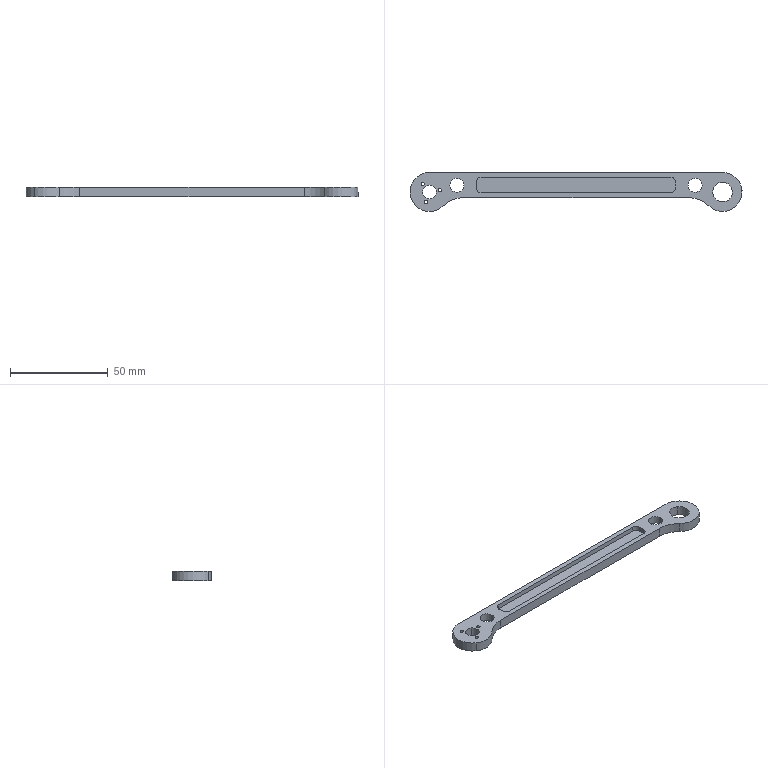Part | NX | features BREP 1 | 1 solid | 43 faces | box 169.999 x 20 x 5 mm | volume 8700 mm3 | cylinder 33 | plane 10 | commonest cylinder face diameters 1.7 x6 5 x6 10 x6 20 x6 7.2 x4 7 x2
STEP:
#1=CARTESIAN_POINT('',(-8.148,-15.081,-8.));
#2=VERTEX_POINT('',#1);
#3=CARTESIAN_POINT('',(-9.848,-15.081,-8.));
#4=VERTEX_POINT('',#3);
#5=CARTESIAN_POINT('',(-8.998,-15.081,-8.));
#6=DIRECTION('',(0.,0.,-1.));
#7=DIRECTION('',(-1.,0.,0.));
#8=AXIS2_PLACEMENT_3D('',#5,#6,#7);
#9=CIRCLE('',#8,0.85);
#10=EDGE_CURVE('',#2,#4,#9,.T.);
#11=ORIENTED_EDGE('',*,*,#10,.T.);
#12=CARTESIAN_POINT('',(-9.848,-15.081,-3.));
#13=VERTEX_POINT('',#12);
#14=CARTESIAN_POINT('',(-9.848,-15.081,-13.));
#15=DIRECTION('',(0.,0.,1.));
#16=VECTOR('',#15,1000.);
#17=LINE('',#14,#16);
#18=EDGE_CURVE('',#4,#13,#17,.T.);
#19=ORIENTED_EDGE('',*,*,#18,.T.);
#20=CARTESIAN_POINT('',(-8.148,-15.081,-3.));
#21=VERTEX_POINT('',#20);
#22=CARTESIAN_POINT('',(-8.998,-15.081,-3.));
#23=DIRECTION('',(0.,0.,1.));
#24=DIRECTION('',(1.,0.,0.));
#25=AXIS2_PLACEMENT_3D('',#22,#23,#24);
#26=CIRCLE('',#25,0.85);
#27=EDGE_CURVE('',#13,#21,#26,.T.);
#28=ORIENTED_EDGE('',*,*,#27,.T.);
#29=CARTESIAN_POINT('',(-8.148,-15.081,-13.));
#30=DIRECTION('',(0.,0.,1.));
#31=VECTOR('',#30,1000.);
#32=LINE('',#29,#31);
#33=EDGE_CURVE('',#2,#21,#32,.T.);
#34=ORIENTED_EDGE('',*,*,#33,.F.);
#35=EDGE_LOOP('',(#11,#19,#28,#34));
#36=FACE_BOUND('',#35,.T.);
#37=CARTESIAN_POINT('',(-8.998,-15.081,-13.));
#38=DIRECTION('',(0.,0.,1.));
#39=DIRECTION('',(-1.,0.,0.));
#40=AXIS2_PLACEMENT_3D('',#37,#38,#39);
#41=CYLINDRICAL_SURFACE('',#40,0.85);
#42=ADVANCED_FACE('',(#36),#41,.F.);
#43=CARTESIAN_POINT('',(-9.816,-5.882,-8.));
#44=VERTEX_POINT('',#43);
#45=CARTESIAN_POINT('',(-11.516,-5.882,-8.));
#46=VERTEX_POINT('',#45);
#47=CARTESIAN_POINT('',(-10.666,-5.882,-8.));
#48=DIRECTION('',(0.,0.,-1.));
#49=DIRECTION('',(-1.,0.,0.));
#50=AXIS2_PLACEMENT_3D('',#47,#48,#49);
#51=CIRCLE('',#50,0.85);
#52=EDGE_CURVE('',#44,#46,#51,.T.);
#53=ORIENTED_EDGE('',*,*,#52,.T.);
#54=CARTESIAN_POINT('',(-11.516,-5.882,-3.));
#55=VERTEX_POINT('',#54);
#56=CARTESIAN_POINT('',(-11.516,-5.882,-13.));
#57=DIRECTION('',(0.,0.,1.));
#58=VECTOR('',#57,1000.);
#59=LINE('',#56,#58);
#60=EDGE_CURVE('',#46,#55,#59,.T.);
#61=ORIENTED_EDGE('',*,*,#60,.T.);
#62=CARTESIAN_POINT('',(-9.816,-5.882,-3.));
#63=VERTEX_POINT('',#62);
#64=CARTESIAN_POINT('',(-10.666,-5.882,-3.));
#65=DIRECTION('',(0.,0.,1.));
#66=DIRECTION('',(1.,0.,0.));
#67=AXIS2_PLACEMENT_3D('',#64,#65,#66);
#68=CIRCLE('',#67,0.85);
#69=EDGE_CURVE('',#55,#63,#68,.T.);
#70=ORIENTED_EDGE('',*,*,#69,.T.);
#71=CARTESIAN_POINT('',(-9.816,-5.882,-13.));
#72=DIRECTION('',(0.,0.,1.));
#73=VECTOR('',#72,1000.);
#74=LINE('',#71,#73);
#75=EDGE_CURVE('',#44,#63,#74,.T.);
#76=ORIENTED_EDGE('',*,*,#75,.F.);
#77=EDGE_LOOP('',(#53,#61,#70,#76));
#78=FACE_BOUND('',#77,.T.);
#79=CARTESIAN_POINT('',(-10.666,-5.882,-13.));
#80=DIRECTION('',(0.,0.,1.));
#81=DIRECTION('',(-1.,0.,0.));
#82=AXIS2_PLACEMENT_3D('',#79,#80,#81);
#83=CYLINDRICAL_SURFACE('',#82,0.85);
#84=ADVANCED_FACE('',(#78),#83,.F.);
#85=CARTESIAN_POINT('',(-1.015,-9.037,-8.));
#86=VERTEX_POINT('',#85);
#87=CARTESIAN_POINT('',(-2.715,-9.037,-8.));
#88=VERTEX_POINT('',#87);
#89=CARTESIAN_POINT('',(-1.865,-9.037,-8.));
#90=DIRECTION('',(0.,0.,-1.));
#91=DIRECTION('',(-1.,0.,0.));
#92=AXIS2_PLACEMENT_3D('',#89,#90,#91);
#93=CIRCLE('',#92,0.85);
#94=EDGE_CURVE('',#86,#88,#93,.T.);
#95=ORIENTED_EDGE('',*,*,#94,.T.);
#96=CARTESIAN_POINT('',(-2.715,-9.037,-3.));
#97=VERTEX_POINT('',#96);
#98=CARTESIAN_POINT('',(-2.715,-9.037,-13.));
#99=DIRECTION('',(0.,0.,1.));
#100=VECTOR('',#99,1000.);
#101=LINE('',#98,#100);
#102=EDGE_CURVE('',#88,#97,#101,.T.);
#103=ORIENTED_EDGE('',*,*,#102,.T.);
#104=CARTESIAN_POINT('',(-1.015,-9.037,-3.));
#105=VERTEX_POINT('',#104);
#106=CARTESIAN_POINT('',(-1.865,-9.037,-3.));
#107=DIRECTION('',(0.,0.,1.));
#108=DIRECTION('',(1.,0.,0.));
#109=AXIS2_PLACEMENT_3D('',#106,#107,#108);
#110=CIRCLE('',#109,0.85);
#111=EDGE_CURVE('',#97,#105,#110,.T.);
#112=ORIENTED_EDGE('',*,*,#111,.T.);
#113=CARTESIAN_POINT('',(-1.015,-9.037,-13.));
#114=DIRECTION('',(0.,0.,1.));
#115=VECTOR('',#114,1000.);
#116=LINE('',#113,#115);
#117=EDGE_CURVE('',#86,#105,#116,.T.);
#118=ORIENTED_EDGE('',*,*,#117,.F.);
#119=EDGE_LOOP('',(#95,#103,#112,#118));
#120=FACE_BOUND('',#119,.T.);
#121=CARTESIAN_POINT('',(-1.865,-9.037,-13.));
#122=DIRECTION('',(0.,0.,1.));
#123=DIRECTION('',(-1.,0.,0.));
#124=AXIS2_PLACEMENT_3D('',#121,#122,#123);
#125=CYLINDRICAL_SURFACE('',#124,0.85);
#126=ADVANCED_FACE('',(#120),#125,.F.);
#127=CARTESIAN_POINT('',(16.824,-6.577,-5.5));
#128=VERTEX_POINT('',#127);
#129=CARTESIAN_POINT('',(16.771,-7.608,-5.5));
#130=VERTEX_POINT('',#129);
#131=CARTESIAN_POINT('',(6.824,-6.577,-5.5));
#132=DIRECTION('',(0.,0.,-1.));
#133=DIRECTION('',(1.,0.,0.));
#134=AXIS2_PLACEMENT_3D('',#131,#132,#133);
#135=CIRCLE('',#134,10.);
#136=EDGE_CURVE('',#128,#130,#135,.T.);
#137=ORIENTED_EDGE('',*,*,#136,.F.);
#138=CARTESIAN_POINT('',(16.824,-6.577,-3.));
#139=VERTEX_POINT('',#138);
#140=CARTESIAN_POINT('',(16.824,-6.577,-5.5));
#141=DIRECTION('',(0.,0.,1.));
#142=VECTOR('',#141,1000.);
#143=LINE('',#140,#142);
#144=EDGE_CURVE('',#128,#139,#143,.T.);
#145=ORIENTED_EDGE('',*,*,#144,.T.);
#146=CARTESIAN_POINT('',(16.771,-7.608,-3.));
#147=VERTEX_POINT('',#146);
#148=CARTESIAN_POINT('',(6.824,-6.577,-3.));
#149=DIRECTION('',(0.,0.,-1.));
#150=DIRECTION('',(1.,0.,0.));
#151=AXIS2_PLACEMENT_3D('',#148,#149,#150);
#152=CIRCLE('',#151,10.);
#153=EDGE_CURVE('',#139,#147,#152,.T.);
#154=ORIENTED_EDGE('',*,*,#153,.T.);
#155=CARTESIAN_POINT('',(16.771,-7.608,-5.5));
#156=DIRECTION('',(0.,0.,1.));
#157=VECTOR('',#156,1000.);
#158=LINE('',#155,#157);
#159=EDGE_CURVE('',#130,#147,#158,.T.);
#160=ORIENTED_EDGE('',*,*,#159,.F.);
#161=EDGE_LOOP('',(#137,#145,#154,#160));
#162=FACE_BOUND('',#161,.T.);
#163=CARTESIAN_POINT('',(6.824,-6.577,-5.5));
#164=DIRECTION('',(0.,0.,1.));
#165=DIRECTION('',(-1.,0.,0.));
#166=AXIS2_PLACEMENT_3D('',#163,#164,#165);
#167=CYLINDRICAL_SURFACE('',#166,10.);
#168=ADVANCED_FACE('',(#162),#167,.T.);
#169=CARTESIAN_POINT('',(118.89,-7.866,-5.5));
#170=VERTEX_POINT('',#169);
#171=CARTESIAN_POINT('',(118.877,-7.608,-5.5));
#172=VERTEX_POINT('',#171);
#173=CARTESIAN_POINT('',(116.39,-7.866,-5.5));
#174=DIRECTION('',(0.,0.,1.));
#175=DIRECTION('',(1.,0.,0.));
#176=AXIS2_PLACEMENT_3D('',#173,#174,#175);
#177=CIRCLE('',#176,2.5);
#178=EDGE_CURVE('',#170,#172,#177,.T.);
#179=ORIENTED_EDGE('',*,*,#178,.F.);
#180=CARTESIAN_POINT('',(118.89,-7.866,-3.));
#181=VERTEX_POINT('',#180);
#182=CARTESIAN_POINT('',(118.89,-7.866,-5.5));
#183=DIRECTION('',(0.,0.,1.));
#184=VECTOR('',#183,1000.);
#185=LINE('',#182,#184);
#186=EDGE_CURVE('',#170,#181,#185,.T.);
#187=ORIENTED_EDGE('',*,*,#186,.T.);
#188=CARTESIAN_POINT('',(118.877,-7.608,-3.));
#189=VERTEX_POINT('',#188);
#190=CARTESIAN_POINT('',(116.39,-7.866,-3.));
#191=DIRECTION('',(0.,0.,1.));
#192=DIRECTION('',(1.,0.,0.));
#193=AXIS2_PLACEMENT_3D('',#190,#191,#192);
#194=CIRCLE('',#193,2.5);
#195=EDGE_CURVE('',#181,#189,#194,.T.);
#196=ORIENTED_EDGE('',*,*,#195,.T.);
#197=CARTESIAN_POINT('',(118.877,-7.608,-5.5));
#198=DIRECTION('',(0.,0.,1.));
#199=VECTOR('',#198,1000.);
#200=LINE('',#197,#199);
#201=EDGE_CURVE('',#172,#189,#200,.T.);
#202=ORIENTED_EDGE('',*,*,#201,.F.);
#203=EDGE_LOOP('',(#179,#187,#196,#202));
#204=FACE_BOUND('',#203,.T.);
#205=CARTESIAN_POINT('',(116.39,-7.866,-5.5));
#206=DIRECTION('',(0.,0.,1.));
#207=DIRECTION('',(-1.,0.,0.));
#208=AXIS2_PLACEMENT_3D('',#205,#206,#207);
#209=CYLINDRICAL_SURFACE('',#208,2.5);
#210=ADVANCED_FACE('',(#204),#209,.F.);
#211=CARTESIAN_POINT('',(118.924,-5.,-5.5));
#212=VERTEX_POINT('',#211);
#213=CARTESIAN_POINT('',(116.424,-2.5,-5.5));
#214=VERTEX_POINT('',#213);
#215=CARTESIAN_POINT('',(116.424,-5.,-5.5));
#216=DIRECTION('',(0.,0.,1.));
#217=DIRECTION('',(1.,0.,0.));
#218=AXIS2_PLACEMENT_3D('',#215,#216,#217);
#219=CIRCLE('',#218,2.5);
#220=EDGE_CURVE('',#212,#214,#219,.T.);
#221=ORIENTED_EDGE('',*,*,#220,.F.);
#222=CARTESIAN_POINT('',(118.924,-5.,-3.));
#223=VERTEX_POINT('',#222);
#224=CARTESIAN_POINT('',(118.924,-5.,-5.5));
#225=DIRECTION('',(0.,0.,1.));
#226=VECTOR('',#225,1000.);
#227=LINE('',#224,#226);
#228=EDGE_CURVE('',#212,#223,#227,.T.);
#229=ORIENTED_EDGE('',*,*,#228,.T.);
#230=CARTESIAN_POINT('',(116.424,-2.5,-3.));
#231=VERTEX_POINT('',#230);
#232=CARTESIAN_POINT('',(116.424,-5.,-3.));
#233=DIRECTION('',(0.,0.,1.));
#234=DIRECTION('',(1.,0.,0.));
#235=AXIS2_PLACEMENT_3D('',#232,#233,#234);
#236=CIRCLE('',#235,2.5);
#237=EDGE_CURVE('',#223,#231,#236,.T.);
#238=ORIENTED_EDGE('',*,*,#237,.T.);
#239=CARTESIAN_POINT('',(116.424,-2.5,-5.5));
#240=DIRECTION('',(0.,0.,1.));
#241=VECTOR('',#240,1000.);
#242=LINE('',#239,#241);
#243=EDGE_CURVE('',#214,#231,#242,.T.);
#244=ORIENTED_EDGE('',*,*,#243,.F.);
#245=EDGE_LOOP('',(#221,#229,#238,#244));
#246=FACE_BOUND('',#245,.T.);
#247=CARTESIAN_POINT('',(116.424,-5.,-5.5));
#248=DIRECTION('',(0.,0.,1.));
#249=DIRECTION('',(-1.,0.,0.));
#250=AXIS2_PLACEMENT_3D('',#247,#248,#249);
#251=CYLINDRICAL_SURFACE('',#250,2.5);
#252=ADVANCED_FACE('',(#246),#251,.F.);
#253=CARTESIAN_POINT('',(11.824,-6.577,-7.));
#254=VERTEX_POINT('',#253);
#255=CARTESIAN_POINT('',(1.824,-6.577,-7.));
#256=VERTEX_POINT('',#255);
#257=CARTESIAN_POINT('',(6.824,-6.577,-7.));
#258=DIRECTION('',(0.,0.,-1.));
#259=DIRECTION('',(-1.,0.,0.));
#260=AXIS2_PLACEMENT_3D('',#257,#258,#259);
#261=CIRCLE('',#260,5.);
#262=EDGE_CURVE('',#254,#256,#261,.T.);
#263=ORIENTED_EDGE('',*,*,#262,.F.);
#264=CARTESIAN_POINT('',(11.824,-6.577,-8.));
#265=VERTEX_POINT('',#264);
#266=CARTESIAN_POINT('',(11.824,-6.577,-7.));
#267=DIRECTION('',(0.,0.,-1.));
#268=VECTOR('',#267,1000.);
#269=LINE('',#266,#268);
#270=EDGE_CURVE('',#265,#254,#269,.F.);
#271=ORIENTED_EDGE('',*,*,#270,.F.);
#272=CARTESIAN_POINT('',(1.824,-6.577,-8.));
#273=VERTEX_POINT('',#272);
#274=CARTESIAN_POINT('',(6.824,-6.577,-8.));
#275=DIRECTION('',(0.,0.,-1.));
#276=DIRECTION('',(-1.,0.,0.));
#277=AXIS2_PLACEMENT_3D('',#274,#275,#276);
#278=CIRCLE('',#277,5.);
#279=EDGE_CURVE('',#265,#273,#278,.T.);
#280=ORIENTED_EDGE('',*,*,#279,.T.);
#281=CARTESIAN_POINT('',(1.824,-6.577,-7.));
#282=DIRECTION('',(0.,0.,-1.));
#283=VECTOR('',#282,1000.);
#284=LINE('',#281,#283);
#285=EDGE_CURVE('',#273,#256,#284,.F.);
#286=ORIENTED_EDGE('',*,*,#285,.T.);
#287=EDGE_LOOP('',(#263,#271,#280,#286));
#288=FACE_BOUND('',#287,.T.);
#289=CARTESIAN_POINT('',(6.824,-6.577,-7.));
#290=DIRECTION('',(0.,0.,-1.));
#291=DIRECTION('',(1.,0.,0.));
#292=AXIS2_PLACEMENT_3D('',#289,#290,#291);
#293=CYLINDRICAL_SURFACE('',#292,5.);
#294=ADVANCED_FACE('',(#288),#293,.F.);
#295=CARTESIAN_POINT('',(133.824,-6.577,-7.));
#296=VERTEX_POINT('',#295);
#297=CARTESIAN_POINT('',(123.824,-6.577,-7.));
#298=VERTEX_POINT('',#297);
#299=CARTESIAN_POINT('',(128.824,-6.577,-7.));
#300=DIRECTION('',(0.,0.,-1.));
#301=DIRECTION('',(-1.,0.,0.));
#302=AXIS2_PLACEMENT_3D('',#299,#300,#301);
#303=CIRCLE('',#302,5.);
#304=EDGE_CURVE('',#296,#298,#303,.T.);
#305=ORIENTED_EDGE('',*,*,#304,.F.);
#306=CARTESIAN_POINT('',(133.824,-6.577,-8.));
#307=VERTEX_POINT('',#306);
#308=CARTESIAN_POINT('',(133.824,-6.577,-7.));
#309=DIRECTION('',(0.,0.,-1.));
#310=VECTOR('',#309,1000.);
#311=LINE('',#308,#310);
#312=EDGE_CURVE('',#307,#296,#311,.F.);
#313=ORIENTED_EDGE('',*,*,#312,.F.);
#314=CARTESIAN_POINT('',(123.824,-6.577,-8.));
#315=VERTEX_POINT('',#314);
#316=CARTESIAN_POINT('',(128.824,-6.577,-8.));
#317=DIRECTION('',(0.,0.,-1.));
#318=DIRECTION('',(-1.,0.,0.));
#319=AXIS2_PLACEMENT_3D('',#316,#317,#318);
#320=CIRCLE('',#319,5.);
#321=EDGE_CURVE('',#307,#315,#320,.T.);
#322=ORIENTED_EDGE('',*,*,#321,.T.);
#323=CARTESIAN_POINT('',(123.824,-6.577,-7.));
#324=DIRECTION('',(0.,0.,-1.));
#325=VECTOR('',#324,1000.);
#326=LINE('',#323,#325);
#327=EDGE_CURVE('',#315,#298,#326,.F.);
#328=ORIENTED_EDGE('',*,*,#327,.T.);
#329=EDGE_LOOP('',(#305,#313,#322,#328));
#330=FACE_BOUND('',#329,.T.);
#331=CARTESIAN_POINT('',(128.824,-6.577,-7.));
#332=DIRECTION('',(0.,0.,-1.));
#333=DIRECTION('',(1.,0.,0.));
#334=AXIS2_PLACEMENT_3D('',#331,#332,#333);
#335=CYLINDRICAL_SURFACE('',#334,5.);
#336=ADVANCED_FACE('',(#330),#335,.F.);
#337=CARTESIAN_POINT('',(145.634,-5.864,-8.));
#338=VERTEX_POINT('',#337);
#339=CARTESIAN_POINT('',(140.014,-14.136,-8.));
#340=VERTEX_POINT('',#339);
#341=CARTESIAN_POINT('',(142.824,-10.,-8.));
#342=DIRECTION('',(0.,0.,1.));
#343=DIRECTION('',(-1.,0.,0.));
#344=AXIS2_PLACEMENT_3D('',#341,#342,#343);
#345=CIRCLE('',#344,5.);
#346=EDGE_CURVE('',#338,#340,#345,.T.);
#347=ORIENTED_EDGE('',*,*,#346,.F.);
#348=CARTESIAN_POINT('',(145.634,-5.864,-3.));
#349=VERTEX_POINT('',#348);
#350=CARTESIAN_POINT('',(145.634,-5.864,-6.));
#351=DIRECTION('',(0.,0.,1.));
#352=VECTOR('',#351,1000.);
#353=LINE('',#350,#352);
#354=EDGE_CURVE('',#349,#338,#353,.F.);
#355=ORIENTED_EDGE('',*,*,#354,.F.);
#356=CARTESIAN_POINT('',(140.014,-14.136,-3.));
#357=VERTEX_POINT('',#356);
#358=CARTESIAN_POINT('',(142.824,-10.,-3.));
#359=DIRECTION('',(0.,0.,1.));
#360=DIRECTION('',(-1.,0.,0.));
#361=AXIS2_PLACEMENT_3D('',#358,#359,#360);
#362=CIRCLE('',#361,5.);
#363=EDGE_CURVE('',#349,#357,#362,.T.);
#364=ORIENTED_EDGE('',*,*,#363,.T.);
#365=CARTESIAN_POINT('',(140.014,-14.136,-6.));
#366=DIRECTION('',(0.,0.,1.));
#367=VECTOR('',#366,1000.);
#368=LINE('',#365,#367);
#369=EDGE_CURVE('',#357,#340,#368,.F.);
#370=ORIENTED_EDGE('',*,*,#369,.T.);
#371=EDGE_LOOP('',(#347,#355,#364,#370));
#372=FACE_BOUND('',#371,.T.);
#373=CARTESIAN_POINT('',(142.824,-10.,-6.));
#374=DIRECTION('',(0.,0.,1.));
#375=DIRECTION('',(0.562,0.8271,0.));
#376=AXIS2_PLACEMENT_3D('',#373,#374,#375);
#377=CYLINDRICAL_SURFACE('',#376,5.);
#378=ADVANCED_FACE('',(#372),#377,.F.);
#379=CARTESIAN_POINT('',(-7.176,0.,-8.));
#380=VERTEX_POINT('',#379);
#381=CARTESIAN_POINT('',(-12.797,-18.271,-8.));
#382=VERTEX_POINT('',#381);
#383=CARTESIAN_POINT('',(-7.176,-10.,-8.));
#384=DIRECTION('',(0.,0.,1.));
#385=DIRECTION('',(-1.,0.,0.));
#386=AXIS2_PLACEMENT_3D('',#383,#384,#385);
#387=CIRCLE('',#386,10.);
#388=EDGE_CURVE('',#380,#382,#387,.T.);
#389=ORIENTED_EDGE('',*,*,#388,.T.);
#390=CARTESIAN_POINT('',(-12.797,-18.271,-3.));
#391=VERTEX_POINT('',#390);
#392=CARTESIAN_POINT('',(-12.797,-18.271,-6.));
#393=DIRECTION('',(0.,0.,1.));
#394=VECTOR('',#393,1000.);
#395=LINE('',#392,#394);
#396=EDGE_CURVE('',#382,#391,#395,.T.);
#397=ORIENTED_EDGE('',*,*,#396,.T.);
#398=CARTESIAN_POINT('',(-7.176,0.,-3.));
#399=VERTEX_POINT('',#398);
#400=CARTESIAN_POINT('',(-7.176,-10.,-3.));
#401=DIRECTION('',(0.,0.,1.));
#402=DIRECTION('',(0.562,0.8271,0.));
#403=AXIS2_PLACEMENT_3D('',#400,#401,#402);
#404=CIRCLE('',#403,10.);
#405=EDGE_CURVE('',#399,#391,#404,.T.);
#406=ORIENTED_EDGE('',*,*,#405,.F.);
#407=CARTESIAN_POINT('',(-7.176,0.,-6.));
#408=DIRECTION('',(0.,0.,1.));
#409=VECTOR('',#408,1000.);
#410=LINE('',#407,#409);
#411=EDGE_CURVE('',#380,#399,#410,.T.);
#412=ORIENTED_EDGE('',*,*,#411,.F.);
#413=EDGE_LOOP('',(#389,#397,#406,#412));
#414=FACE_BOUND('',#413,.T.);
#415=CARTESIAN_POINT('',(-7.176,-10.,-6.));
#416=DIRECTION('',(0.,0.,1.));
#417=DIRECTION('',(0.562,0.8271,0.));
#418=AXIS2_PLACEMENT_3D('',#415,#416,#417);
#419=CYLINDRICAL_SURFACE('',#418,10.);
#420=ADVANCED_FACE('',(#414),#419,.T.);
#421=CARTESIAN_POINT('',(-5.209,-7.105,-8.));
#422=VERTEX_POINT('',#421);
#423=CARTESIAN_POINT('',(-9.143,-12.895,-8.));
#424=VERTEX_POINT('',#423);
#425=CARTESIAN_POINT('',(-7.176,-10.,-8.));
#426=DIRECTION('',(0.,0.,1.));
#427=DIRECTION('',(-1.,0.,0.));
#428=AXIS2_PLACEMENT_3D('',#425,#426,#427);
#429=CIRCLE('',#428,3.5);
#430=EDGE_CURVE('',#422,#424,#429,.T.);
#431=ORIENTED_EDGE('',*,*,#430,.F.);
#432=CARTESIAN_POINT('',(-5.209,-7.105,-3.));
#433=VERTEX_POINT('',#432);
#434=CARTESIAN_POINT('',(-5.209,-7.105,-6.));
#435=DIRECTION('',(0.,0.,1.));
#436=VECTOR('',#435,1000.);
#437=LINE('',#434,#436);
#438=EDGE_CURVE('',#433,#422,#437,.F.);
#439=ORIENTED_EDGE('',*,*,#438,.F.);
#440=CARTESIAN_POINT('',(-9.143,-12.895,-3.));
#441=VERTEX_POINT('',#440);
#442=CARTESIAN_POINT('',(-7.176,-10.,-3.));
#443=DIRECTION('',(0.,0.,1.));
#444=DIRECTION('',(-1.,0.,0.));
#445=AXIS2_PLACEMENT_3D('',#442,#443,#444);
#446=CIRCLE('',#445,3.5);
#447=EDGE_CURVE('',#433,#441,#446,.T.);
#448=ORIENTED_EDGE('',*,*,#447,.T.);
#449=CARTESIAN_POINT('',(-9.143,-12.895,-6.));
#450=DIRECTION('',(0.,0.,1.));
#451=VECTOR('',#450,1000.);
#452=LINE('',#449,#451);
#453=EDGE_CURVE('',#441,#424,#452,.F.);
#454=ORIENTED_EDGE('',*,*,#453,.T.);
#455=EDGE_LOOP('',(#431,#439,#448,#454));
#456=FACE_BOUND('',#455,.T.);
#457=CARTESIAN_POINT('',(-7.176,-10.,-6.));
#458=DIRECTION('',(0.,0.,1.));
#459=DIRECTION('',(0.562,0.8271,0.));
#460=AXIS2_PLACEMENT_3D('',#457,#458,#459);
#461=CYLINDRICAL_SURFACE('',#460,3.5);
#462=ADVANCED_FACE('',(#456),#461,.F.);
#463=CARTESIAN_POINT('',(132.424,-6.577,-3.));
#464=VERTEX_POINT('',#463);
#465=CARTESIAN_POINT('',(125.224,-6.577,-3.));
#466=VERTEX_POINT('',#465);
#467=CARTESIAN_POINT('',(128.824,-6.577,-3.));
#468=DIRECTION('',(0.,0.,-1.));
#469=DIRECTION('',(-1.,0.,0.));
#470=AXIS2_PLACEMENT_3D('',#467,#468,#469);
#471=CIRCLE('',#470,3.6);
#472=EDGE_CURVE('',#464,#466,#471,.T.);
#473=ORIENTED_EDGE('',*,*,#472,.F.);
#474=CARTESIAN_POINT('',(132.424,-6.577,-7.));
#475=VERTEX_POINT('',#474);
#476=CARTESIAN_POINT('',(132.424,-6.577,28.));
#477=DIRECTION('',(0.,0.,-1.));
#478=VECTOR('',#477,1000.);
#479=LINE('',#476,#478);
#480=EDGE_CURVE('',#475,#464,#479,.F.);
#481=ORIENTED_EDGE('',*,*,#480,.F.);
#482=CARTESIAN_POINT('',(125.224,-6.577,-7.));
#483=VERTEX_POINT('',#482);
#484=CARTESIAN_POINT('',(128.824,-6.577,-7.));
#485=DIRECTION('',(0.,0.,1.));
#486=DIRECTION('',(-1.,0.,0.));
#487=AXIS2_PLACEMENT_3D('',#484,#485,#486);
#488=CIRCLE('',#487,3.6);
#489=EDGE_CURVE('',#483,#475,#488,.T.);
#490=ORIENTED_EDGE('',*,*,#489,.F.);
#491=CARTESIAN_POINT('',(125.224,-6.577,28.));
#492=DIRECTION('',(0.,0.,-1.));
#493=VECTOR('',#492,1000.);
#494=LINE('',#491,#493);
#495=EDGE_CURVE('',#483,#466,#494,.F.);
#496=ORIENTED_EDGE('',*,*,#495,.T.);
#497=EDGE_LOOP('',(#473,#481,#490,#496));
#498=FACE_BOUND('',#497,.T.);
#499=CARTESIAN_POINT('',(128.824,-6.577,28.));
#500=DIRECTION('',(0.,0.,-1.));
#501=DIRECTION('',(1.,0.,0.));
#502=AXIS2_PLACEMENT_3D('',#499,#500,#501);
#503=CYLINDRICAL_SURFACE('',#502,3.6);
#504=ADVANCED_FACE('',(#498),#503,.F.);
#505=CARTESIAN_POINT('',(10.424,-6.577,-3.));
#506=VERTEX_POINT('',#505);
#507=CARTESIAN_POINT('',(3.224,-6.577,-3.));
#508=VERTEX_POINT('',#507);
#509=CARTESIAN_POINT('',(6.824,-6.577,-3.));
#510=DIRECTION('',(0.,0.,-1.));
#511=DIRECTION('',(-1.,0.,0.));
#512=AXIS2_PLACEMENT_3D('',#509,#510,#511);
#513=CIRCLE('',#512,3.6);
#514=EDGE_CURVE('',#506,#508,#513,.T.);
#515=ORIENTED_EDGE('',*,*,#514,.F.);
#516=CARTESIAN_POINT('',(10.424,-6.577,-7.));
#517=VERTEX_POINT('',#516);
#518=CARTESIAN_POINT('',(10.424,-6.577,28.));
#519=DIRECTION('',(0.,0.,-1.));
#520=VECTOR('',#519,1000.);
#521=LINE('',#518,#520);
#522=EDGE_CURVE('',#517,#506,#521,.F.);
#523=ORIENTED_EDGE('',*,*,#522,.F.);
#524=CARTESIAN_POINT('',(3.224,-6.577,-7.));
#525=VERTEX_POINT('',#524);
#526=CARTESIAN_POINT('',(6.824,-6.577,-7.));
#527=DIRECTION('',(0.,0.,1.));
#528=DIRECTION('',(-1.,0.,0.));
#529=AXIS2_PLACEMENT_3D('',#526,#527,#528);
#530=CIRCLE('',#529,3.6);
#531=EDGE_CURVE('',#525,#517,#530,.T.);
#532=ORIENTED_EDGE('',*,*,#531,.F.);
#533=CARTESIAN_POINT('',(3.224,-6.577,28.));
#534=DIRECTION('',(0.,0.,-1.));
#535=VECTOR('',#534,1000.);
#536=LINE('',#533,#535);
#537=EDGE_CURVE('',#525,#508,#536,.F.);
#538=ORIENTED_EDGE('',*,*,#537,.T.);
#539=EDGE_LOOP('',(#515,#523,#532,#538));
#540=FACE_BOUND('',#539,.T.);
#541=CARTESIAN_POINT('',(6.824,-6.577,28.));
#542=DIRECTION('',(0.,0.,-1.));
#543=DIRECTION('',(1.,0.,0.));
#544=AXIS2_PLACEMENT_3D('',#541,#542,#543);
#545=CYLINDRICAL_SURFACE('',#544,3.6);
#546=ADVANCED_FACE('',(#540),#545,.F.);
#547=ORIENTED_EDGE('',*,*,#522,.T.);
#548=CARTESIAN_POINT('',(6.824,-6.577,-3.));
#549=DIRECTION('',(0.,0.,-1.));
#550=DIRECTION('',(-1.,0.,0.));
#551=AXIS2_PLACEMENT_3D('',#548,#549,#550);
#552=CIRCLE('',#551,3.6);
#553=EDGE_CURVE('',#508,#506,#552,.T.);
#554=ORIENTED_EDGE('',*,*,#553,.F.);
#555=ORIENTED_EDGE('',*,*,#537,.F.);
#556=CARTESIAN_POINT('',(6.824,-6.577,-7.));
#557=DIRECTION('',(0.,0.,1.));
#558=DIRECTION('',(-1.,0.,0.));
#559=AXIS2_PLACEMENT_3D('',#556,#557,#558);
#560=CIRCLE('',#559,3.6);
#561=EDGE_CURVE('',#517,#525,#560,.T.);
#562=ORIENTED_EDGE('',*,*,#561,.F.);
#563=EDGE_LOOP('',(#547,#554,#555,#562));
#564=FACE_BOUND('',#563,.T.);
#565=CARTESIAN_POINT('',(6.824,-6.577,28.));
#566=DIRECTION('',(0.,0.,-1.));
#567=DIRECTION('',(1.,0.,0.));
#568=AXIS2_PLACEMENT_3D('',#565,#566,#567);
#569=CYLINDRICAL_SURFACE('',#568,3.6);
#570=ADVANCED_FACE('',(#564),#569,.F.);
#571=ORIENTED_EDGE('',*,*,#480,.T.);
#572=CARTESIAN_POINT('',(128.824,-6.577,-3.));
#573=DIRECTION('',(0.,0.,-1.));
#574=DIRECTION('',(-1.,0.,0.));
#575=AXIS2_PLACEMENT_3D('',#572,#573,#574);
#576=CIRCLE('',#575,3.6);
#577=EDGE_CURVE('',#466,#464,#576,.T.);
#578=ORIENTED_EDGE('',*,*,#577,.F.);
#579=ORIENTED_EDGE('',*,*,#495,.F.);
#580=CARTESIAN_POINT('',(128.824,-6.577,-7.));
#581=DIRECTION('',(0.,0.,1.));
#582=DIRECTION('',(-1.,0.,0.));
#583=AXIS2_PLACEMENT_3D('',#580,#581,#582);
#584=CIRCLE('',#583,3.6);
#585=EDGE_CURVE('',#475,#483,#584,.T.);
#586=ORIENTED_EDGE('',*,*,#585,.F.);
#587=EDGE_LOOP('',(#571,#578,#579,#586));
#588=FACE_BOUND('',#587,.T.);
#589=CARTESIAN_POINT('',(128.824,-6.577,28.));
#590=DIRECTION('',(0.,0.,-1.));
#591=DIRECTION('',(1.,0.,0.));
#592=AXIS2_PLACEMENT_3D('',#589,#590,#591);
#593=CYLINDRICAL_SURFACE('',#592,3.6);
#594=ADVANCED_FACE('',(#588),#593,.F.);
#595=CARTESIAN_POINT('',(-0.1812,-17.146,-8.));
#596=VERTEX_POINT('',#595);
#597=CARTESIAN_POINT('',(10.311,-12.866,-8.));
#598=VERTEX_POINT('',#597);
#599=CARTESIAN_POINT('',(10.311,-27.866,-8.));
#600=DIRECTION('',(0.,0.,-1.));
#601=DIRECTION('',(-1.,0.,0.));
#602=AXIS2_PLACEMENT_3D('',#599,#600,#601);
#603=CIRCLE('',#602,15.);
#604=EDGE_CURVE('',#596,#598,#603,.T.);
#605=ORIENTED_EDGE('',*,*,#604,.F.);
#606=CARTESIAN_POINT('',(-7.176,-10.,-8.));
#607=DIRECTION('',(0.,0.,1.));
#608=DIRECTION('',(-1.,0.,0.));
#609=AXIS2_PLACEMENT_3D('',#606,#607,#608);
#610=CIRCLE('',#609,10.);
#611=EDGE_CURVE('',#382,#596,#610,.T.);
#612=ORIENTED_EDGE('',*,*,#611,.F.);
#613=ORIENTED_EDGE('',*,*,#388,.F.);
#614=CARTESIAN_POINT('',(142.824,0.,-8.));
#615=VERTEX_POINT('',#614);
#616=CARTESIAN_POINT('',(2.824,0.,-8.));
#617=DIRECTION('',(-1.,0.,0.));
#618=VECTOR('',#617,1000.);
#619=LINE('',#616,#618);
#620=EDGE_CURVE('',#615,#380,#619,.T.);
#621=ORIENTED_EDGE('',*,*,#620,.F.);
#622=CARTESIAN_POINT('',(147.956,-1.417,-8.));
#623=VERTEX_POINT('',#622);
#624=CARTESIAN_POINT('',(142.824,-10.,-8.));
#625=DIRECTION('',(0.,0.,1.));
#626=DIRECTION('',(-1.,0.,0.));
#627=AXIS2_PLACEMENT_3D('',#624,#625,#626);
#628=CIRCLE('',#627,10.);
#629=EDGE_CURVE('',#623,#615,#628,.T.);
#630=ORIENTED_EDGE('',*,*,#629,.F.);
#631=CARTESIAN_POINT('',(147.954,-1.418,-8.));
#632=VERTEX_POINT('',#631);
#633=CARTESIAN_POINT('',(166.688,0.,-8.));
#634=DIRECTION('',(0.9971,0.07545,0.));
#635=VECTOR('',#634,1000.);
#636=LINE('',#633,#635);
#637=EDGE_CURVE('',#632,#623,#636,.T.);
#638=ORIENTED_EDGE('',*,*,#637,.F.);
#639=CARTESIAN_POINT('',(135.829,-17.146,-8.));
#640=VERTEX_POINT('',#639);
#641=CARTESIAN_POINT('',(142.823,-10.,-8.));
#642=DIRECTION('',(0.,0.,1.));
#643=DIRECTION('',(-1.,0.,0.));
#644=AXIS2_PLACEMENT_3D('',#641,#642,#643);
#645=CIRCLE('',#644,9.999);
#646=EDGE_CURVE('',#640,#632,#645,.T.);
#647=ORIENTED_EDGE('',*,*,#646,.F.);
#648=CARTESIAN_POINT('',(125.337,-12.866,-8.));
#649=VERTEX_POINT('',#648);
#650=CARTESIAN_POINT('',(125.337,-27.866,-8.));
#651=DIRECTION('',(0.,0.,-1.));
#652=DIRECTION('',(-1.,0.,0.));
#653=AXIS2_PLACEMENT_3D('',#650,#651,#652);
#654=CIRCLE('',#653,15.);
#655=EDGE_CURVE('',#649,#640,#654,.T.);
#656=ORIENTED_EDGE('',*,*,#655,.F.);
#657=CARTESIAN_POINT('',(10.311,-12.866,-8.));
#658=DIRECTION('',(1.,0.000002877,0.));
#659=VECTOR('',#658,1000.);
#660=LINE('',#657,#659);
#661=EDGE_CURVE('',#598,#649,#660,.T.);
#662=ORIENTED_EDGE('',*,*,#661,.F.);
#663=EDGE_LOOP('',(#605,#612,#613,#621,#630,#638,#647,#656,#662));
#664=FACE_BOUND('',#663,.T.);
#665=ORIENTED_EDGE('',*,*,#10,.F.);
#666=CARTESIAN_POINT('',(-8.998,-15.081,-8.));
#667=DIRECTION('',(0.,0.,-1.));
#668=DIRECTION('',(-1.,0.,0.));
#669=AXIS2_PLACEMENT_3D('',#666,#667,#668);
#670=CIRCLE('',#669,0.85);
#671=EDGE_CURVE('',#4,#2,#670,.T.);
#672=ORIENTED_EDGE('',*,*,#671,.F.);
#673=EDGE_LOOP('',(#665,#672));
#674=FACE_BOUND('',#673,.T.);
#675=ORIENTED_EDGE('',*,*,#52,.F.);
#676=CARTESIAN_POINT('',(-10.666,-5.882,-8.));
#677=DIRECTION('',(0.,0.,-1.));
#678=DIRECTION('',(-1.,0.,0.));
#679=AXIS2_PLACEMENT_3D('',#676,#677,#678);
#680=CIRCLE('',#679,0.85);
#681=EDGE_CURVE('',#46,#44,#680,.T.);
#682=ORIENTED_EDGE('',*,*,#681,.F.);
#683=EDGE_LOOP('',(#675,#682));
#684=FACE_BOUND('',#683,.T.);
#685=ORIENTED_EDGE('',*,*,#94,.F.);
#686=CARTESIAN_POINT('',(-1.865,-9.037,-8.));
#687=DIRECTION('',(0.,0.,-1.));
#688=DIRECTION('',(-1.,0.,0.));
#689=AXIS2_PLACEMENT_3D('',#686,#687,#688);
#690=CIRCLE('',#689,0.85);
#691=EDGE_CURVE('',#88,#86,#690,.T.);
#692=ORIENTED_EDGE('',*,*,#691,.F.);
#693=EDGE_LOOP('',(#685,#692));
#694=FACE_BOUND('',#693,.T.);
#695=CARTESIAN_POINT('',(128.824,-6.577,-8.));
#696=DIRECTION('',(0.,0.,-1.));
#697=DIRECTION('',(-1.,0.,0.));
#698=AXIS2_PLACEMENT_3D('',#695,#696,#697);
#699=CIRCLE('',#698,5.);
#700=EDGE_CURVE('',#315,#307,#699,.T.);
#701=ORIENTED_EDGE('',*,*,#700,.F.);
#702=ORIENTED_EDGE('',*,*,#321,.F.);
#703=EDGE_LOOP('',(#701,#702));
#704=FACE_BOUND('',#703,.T.);
#705=CARTESIAN_POINT('',(6.824,-6.577,-8.));
#706=DIRECTION('',(0.,0.,-1.));
#707=DIRECTION('',(-1.,0.,0.));
#708=AXIS2_PLACEMENT_3D('',#705,#706,#707);
#709=CIRCLE('',#708,5.);
#710=EDGE_CURVE('',#273,#265,#709,.T.);
#711=ORIENTED_EDGE('',*,*,#710,.F.);
#712=ORIENTED_EDGE('',*,*,#279,.F.);
#713=EDGE_LOOP('',(#711,#712));
#714=FACE_BOUND('',#713,.T.);
#715=CARTESIAN_POINT('',(142.824,-10.,-8.));
#716=DIRECTION('',(0.,0.,1.));
#717=DIRECTION('',(-1.,0.,0.));
#718=AXIS2_PLACEMENT_3D('',#715,#716,#717);
#719=CIRCLE('',#718,5.);
#720=EDGE_CURVE('',#340,#338,#719,.T.);
#721=ORIENTED_EDGE('',*,*,#720,.T.);
#722=ORIENTED_EDGE('',*,*,#346,.T.);
#723=EDGE_LOOP('',(#721,#722));
#724=FACE_BOUND('',#723,.T.);
#725=CARTESIAN_POINT('',(-7.176,-10.,-8.));
#726=DIRECTION('',(0.,0.,1.));
#727=DIRECTION('',(-1.,0.,0.));
#728=AXIS2_PLACEMENT_3D('',#725,#726,#727);
#729=CIRCLE('',#728,3.5);
#730=EDGE_CURVE('',#424,#422,#729,.T.);
#731=ORIENTED_EDGE('',*,*,#730,.T.);
#732=ORIENTED_EDGE('',*,*,#430,.T.);
#733=EDGE_LOOP('',(#731,#732));
#734=FACE_BOUND('',#733,.T.);
#735=CARTESIAN_POINT('',(2.824,-10.,-8.));
#736=DIRECTION('',(0.,0.,-1.));
#737=DIRECTION('',(0.,1.,0.));
#738=AXIS2_PLACEMENT_3D('',#735,#736,#737);
#739=PLANE('',#738);
#740=ADVANCED_FACE('',(#664,#674,#684,#694,#704,#714,#724,#734),#739,.T.);
#741=ORIENTED_EDGE('',*,*,#405,.T.);
#742=CARTESIAN_POINT('',(-0.1812,-17.146,-3.));
#743=VERTEX_POINT('',#742);
#744=CARTESIAN_POINT('',(-7.176,-10.,-3.));
#745=DIRECTION('',(0.,0.,1.));
#746=DIRECTION('',(0.562,0.8271,0.));
#747=AXIS2_PLACEMENT_3D('',#744,#745,#746);
#748=CIRCLE('',#747,10.);
#749=EDGE_CURVE('',#391,#743,#748,.T.);
#750=ORIENTED_EDGE('',*,*,#749,.T.);
#751=CARTESIAN_POINT('',(10.311,-12.866,-3.));
#752=VERTEX_POINT('',#751);
#753=CARTESIAN_POINT('',(10.311,-27.866,-3.));
#754=DIRECTION('',(0.,0.,-1.));
#755=DIRECTION('',(-1.,0.,0.));
#756=AXIS2_PLACEMENT_3D('',#753,#754,#755);
#757=CIRCLE('',#756,15.);
#758=EDGE_CURVE('',#743,#752,#757,.T.);
#759=ORIENTED_EDGE('',*,*,#758,.T.);
#760=CARTESIAN_POINT('',(125.337,-12.866,-3.));
#761=VERTEX_POINT('',#760);
#762=CARTESIAN_POINT('',(10.311,-12.866,-3.));
#763=DIRECTION('',(1.,0.000002877,0.));
#764=VECTOR('',#763,1000.);
#765=LINE('',#762,#764);
#766=EDGE_CURVE('',#752,#761,#765,.T.);
#767=ORIENTED_EDGE('',*,*,#766,.T.);
#768=CARTESIAN_POINT('',(135.829,-17.146,-3.));
#769=VERTEX_POINT('',#768);
#770=CARTESIAN_POINT('',(125.337,-27.866,-3.));
#771=DIRECTION('',(0.,0.,-1.));
#772=DIRECTION('',(-1.,0.,0.));
#773=AXIS2_PLACEMENT_3D('',#770,#771,#772);
#774=CIRCLE('',#773,15.);
#775=EDGE_CURVE('',#761,#769,#774,.T.);
#776=ORIENTED_EDGE('',*,*,#775,.T.);
#777=CARTESIAN_POINT('',(147.954,-1.418,-3.));
#778=VERTEX_POINT('',#777);
#779=CARTESIAN_POINT('',(142.823,-10.,-3.));
#780=DIRECTION('',(0.,0.,1.));
#781=DIRECTION('',(-1.,0.,0.));
#782=AXIS2_PLACEMENT_3D('',#779,#780,#781);
#783=CIRCLE('',#782,9.999);
#784=EDGE_CURVE('',#769,#778,#783,.T.);
#785=ORIENTED_EDGE('',*,*,#784,.T.);
#786=CARTESIAN_POINT('',(147.956,-1.417,-3.));
#787=VERTEX_POINT('',#786);
#788=CARTESIAN_POINT('',(166.688,0.,-3.));
#789=DIRECTION('',(0.9971,0.07545,0.));
#790=VECTOR('',#789,1000.);
#791=LINE('',#788,#790);
#792=EDGE_CURVE('',#778,#787,#791,.T.);
#793=ORIENTED_EDGE('',*,*,#792,.T.);
#794=CARTESIAN_POINT('',(142.824,0.,-3.));
#795=VERTEX_POINT('',#794);
#796=CARTESIAN_POINT('',(142.824,-10.,-3.));
#797=DIRECTION('',(0.,0.,1.));
#798=DIRECTION('',(0.562,0.8271,0.));
#799=AXIS2_PLACEMENT_3D('',#796,#797,#798);
#800=CIRCLE('',#799,10.);
#801=EDGE_CURVE('',#787,#795,#800,.T.);
#802=ORIENTED_EDGE('',*,*,#801,.T.);
#803=CARTESIAN_POINT('',(2.824,0.,-3.));
#804=DIRECTION('',(-1.,0.,0.));
#805=VECTOR('',#804,1000.);
#806=LINE('',#803,#805);
#807=EDGE_CURVE('',#795,#399,#806,.T.);
#808=ORIENTED_EDGE('',*,*,#807,.T.);
#809=EDGE_LOOP('',(#741,#750,#759,#767,#776,#785,#793,#802,#808));
#810=FACE_BOUND('',#809,.T.);
#811=CARTESIAN_POINT('',(-8.998,-15.081,-3.));
#812=DIRECTION('',(0.,0.,1.));
#813=DIRECTION('',(1.,0.,0.));
#814=AXIS2_PLACEMENT_3D('',#811,#812,#813);
#815=CIRCLE('',#814,0.85);
#816=EDGE_CURVE('',#21,#13,#815,.T.);
#817=ORIENTED_EDGE('',*,*,#816,.F.);
#818=ORIENTED_EDGE('',*,*,#27,.F.);
#819=EDGE_LOOP('',(#817,#818));
#820=FACE_BOUND('',#819,.T.);
#821=CARTESIAN_POINT('',(-10.666,-5.882,-3.));
#822=DIRECTION('',(0.,0.,1.));
#823=DIRECTION('',(1.,0.,0.));
#824=AXIS2_PLACEMENT_3D('',#821,#822,#823);
#825=CIRCLE('',#824,0.85);
#826=EDGE_CURVE('',#63,#55,#825,.T.);
#827=ORIENTED_EDGE('',*,*,#826,.F.);
#828=ORIENTED_EDGE('',*,*,#69,.F.);
#829=EDGE_LOOP('',(#827,#828));
#830=FACE_BOUND('',#829,.T.);
#831=CARTESIAN_POINT('',(-1.865,-9.037,-3.));
#832=DIRECTION('',(0.,0.,1.));
#833=DIRECTION('',(1.,0.,0.));
#834=AXIS2_PLACEMENT_3D('',#831,#832,#833);
#835=CIRCLE('',#834,0.85);
#836=EDGE_CURVE('',#105,#97,#835,.T.);
#837=ORIENTED_EDGE('',*,*,#836,.F.);
#838=ORIENTED_EDGE('',*,*,#111,.F.);
#839=EDGE_LOOP('',(#837,#838));
#840=FACE_BOUND('',#839,.T.);
#841=CARTESIAN_POINT('',(19.224,-2.5,-3.));
#842=VERTEX_POINT('',#841);
#843=CARTESIAN_POINT('',(116.424,-2.5,-3.));
#844=DIRECTION('',(-1.,0.,0.));
#845=VECTOR('',#844,1000.);
#846=LINE('',#843,#845);
#847=EDGE_CURVE('',#231,#842,#846,.T.);
#848=ORIENTED_EDGE('',*,*,#847,.F.);
#849=ORIENTED_EDGE('',*,*,#237,.F.);
#850=CARTESIAN_POINT('',(118.904,-5.315,-3.));
#851=VERTEX_POINT('',#850);
#852=CARTESIAN_POINT('',(116.424,-5.,-3.));
#853=DIRECTION('',(0.,0.,1.));
#854=DIRECTION('',(1.,0.,0.));
#855=AXIS2_PLACEMENT_3D('',#852,#853,#854);
#856=CIRCLE('',#855,2.5);
#857=EDGE_CURVE('',#851,#223,#856,.T.);
#858=ORIENTED_EDGE('',*,*,#857,.F.);
#859=CARTESIAN_POINT('',(128.824,-6.577,-3.));
#860=DIRECTION('',(0.,0.,-1.));
#861=DIRECTION('',(1.,0.,0.));
#862=AXIS2_PLACEMENT_3D('',#859,#860,#861);
#863=CIRCLE('',#862,10.);
#864=EDGE_CURVE('',#189,#851,#863,.T.);
#865=ORIENTED_EDGE('',*,*,#864,.F.);
#866=ORIENTED_EDGE('',*,*,#195,.F.);
#867=CARTESIAN_POINT('',(116.39,-10.366,-3.));
#868=VERTEX_POINT('',#867);
#869=CARTESIAN_POINT('',(116.39,-7.866,-3.));
#870=DIRECTION('',(0.,0.,1.));
#871=DIRECTION('',(1.,0.,0.));
#872=AXIS2_PLACEMENT_3D('',#869,#870,#871);
#873=CIRCLE('',#872,2.5);
#874=EDGE_CURVE('',#868,#181,#873,.T.);
#875=ORIENTED_EDGE('',*,*,#874,.F.);
#876=CARTESIAN_POINT('',(19.257,-10.366,-3.));
#877=VERTEX_POINT('',#876);
#878=CARTESIAN_POINT('',(19.257,-10.366,-3.));
#879=DIRECTION('',(1.,0.000002877,0.));
#880=VECTOR('',#879,1000.);
#881=LINE('',#878,#880);
#882=EDGE_CURVE('',#877,#868,#881,.T.);
#883=ORIENTED_EDGE('',*,*,#882,.F.);
#884=CARTESIAN_POINT('',(19.257,-7.866,-3.));
#885=DIRECTION('',(0.,0.,1.));
#886=DIRECTION('',(-1.,0.,0.));
#887=AXIS2_PLACEMENT_3D('',#884,#885,#886);
#888=CIRCLE('',#887,2.5);
#889=EDGE_CURVE('',#147,#877,#888,.T.);
#890=ORIENTED_EDGE('',*,*,#889,.F.);
#891=ORIENTED_EDGE('',*,*,#153,.F.);
#892=CARTESIAN_POINT('',(16.744,-5.315,-3.));
#893=VERTEX_POINT('',#892);
#894=CARTESIAN_POINT('',(6.824,-6.577,-3.));
#895=DIRECTION('',(0.,0.,-1.));
#896=DIRECTION('',(1.,0.,0.));
#897=AXIS2_PLACEMENT_3D('',#894,#895,#896);
#898=CIRCLE('',#897,10.);
#899=EDGE_CURVE('',#893,#139,#898,.T.);
#900=ORIENTED_EDGE('',*,*,#899,.F.);
#901=CARTESIAN_POINT('',(19.224,-5.,-3.));
#902=DIRECTION('',(0.,0.,1.));
#903=DIRECTION('',(-1.,0.,0.));
#904=AXIS2_PLACEMENT_3D('',#901,#902,#903);
#905=CIRCLE('',#904,2.5);
#906=EDGE_CURVE('',#842,#893,#905,.T.);
#907=ORIENTED_EDGE('',*,*,#906,.F.);
#908=EDGE_LOOP('',(#848,#849,#858,#865,#866,#875,#883,#890,#891,#900,#907));
#909=FACE_BOUND('',#908,.T.);
#910=CARTESIAN_POINT('',(-7.176,-10.,-3.));
#911=DIRECTION('',(0.,0.,1.));
#912=DIRECTION('',(-1.,0.,0.));
#913=AXIS2_PLACEMENT_3D('',#910,#911,#912);
#914=CIRCLE('',#913,3.5);
#915=EDGE_CURVE('',#441,#433,#914,.T.);
#916=ORIENTED_EDGE('',*,*,#915,.F.);
#917=ORIENTED_EDGE('',*,*,#447,.F.);
#918=EDGE_LOOP('',(#916,#917));
#919=FACE_BOUND('',#918,.T.);
#920=CARTESIAN_POINT('',(142.824,-10.,-3.));
#921=DIRECTION('',(0.,0.,1.));
#922=DIRECTION('',(-1.,0.,0.));
#923=AXIS2_PLACEMENT_3D('',#920,#921,#922);
#924=CIRCLE('',#923,5.);
#925=EDGE_CURVE('',#357,#349,#924,.T.);
#926=ORIENTED_EDGE('',*,*,#925,.F.);
#927=ORIENTED_EDGE('',*,*,#363,.F.);
#928=EDGE_LOOP('',(#926,#927));
#929=FACE_BOUND('',#928,.T.);
#930=ORIENTED_EDGE('',*,*,#553,.T.);
#931=ORIENTED_EDGE('',*,*,#514,.T.);
#932=EDGE_LOOP('',(#930,#931));
#933=FACE_BOUND('',#932,.T.);
#934=ORIENTED_EDGE('',*,*,#577,.T.);
#935=ORIENTED_EDGE('',*,*,#472,.T.);
#936=EDGE_LOOP('',(#934,#935));
#937=FACE_BOUND('',#936,.T.);
#938=CARTESIAN_POINT('',(2.824,-10.,-3.));
#939=DIRECTION('',(0.,0.,-1.));
#940=DIRECTION('',(0.,1.,0.));
#941=AXIS2_PLACEMENT_3D('',#938,#939,#940);
#942=PLANE('',#941);
#943=ADVANCED_FACE('',(#810,#820,#830,#840,#909,#919,#929,#933,#937),#942,.F.);
#944=ORIENTED_EDGE('',*,*,#438,.T.);
#945=ORIENTED_EDGE('',*,*,#730,.F.);
#946=ORIENTED_EDGE('',*,*,#453,.F.);
#947=ORIENTED_EDGE('',*,*,#915,.T.);
#948=EDGE_LOOP('',(#944,#945,#946,#947));
#949=FACE_BOUND('',#948,.T.);
#950=CARTESIAN_POINT('',(-7.176,-10.,-6.));
#951=DIRECTION('',(0.,0.,1.));
#952=DIRECTION('',(0.562,0.8271,0.));
#953=AXIS2_PLACEMENT_3D('',#950,#951,#952);
#954=CYLINDRICAL_SURFACE('',#953,3.5);
#955=ADVANCED_FACE('',(#949),#954,.F.);
#956=ORIENTED_EDGE('',*,*,#801,.F.);
#957=CARTESIAN_POINT('',(147.956,-1.417,-6.));
#958=DIRECTION('',(0.,0.,-1.));
#959=VECTOR('',#958,1000.);
#960=LINE('',#957,#959);
#961=EDGE_CURVE('',#787,#623,#960,.T.);
#962=ORIENTED_EDGE('',*,*,#961,.T.);
#963=ORIENTED_EDGE('',*,*,#629,.T.);
#964=CARTESIAN_POINT('',(142.824,0.,-6.));
#965=DIRECTION('',(0.,0.,1.));
#966=VECTOR('',#965,1000.);
#967=LINE('',#964,#966);
#968=EDGE_CURVE('',#615,#795,#967,.T.);
#969=ORIENTED_EDGE('',*,*,#968,.T.);
#970=EDGE_LOOP('',(#956,#962,#963,#969));
#971=FACE_BOUND('',#970,.T.);
#972=CARTESIAN_POINT('',(142.824,-10.,-6.));
#973=DIRECTION('',(0.,0.,1.));
#974=DIRECTION('',(0.562,0.8271,0.));
#975=AXIS2_PLACEMENT_3D('',#972,#973,#974);
#976=CYLINDRICAL_SURFACE('',#975,10.);
#977=ADVANCED_FACE('',(#971),#976,.T.);
#978=ORIENTED_EDGE('',*,*,#396,.F.);
#979=ORIENTED_EDGE('',*,*,#611,.T.);
#980=CARTESIAN_POINT('',(-0.1812,-17.146,-3.));
#981=DIRECTION('',(0.,0.,-1.));
#982=VECTOR('',#981,1000.);
#983=LINE('',#980,#982);
#984=EDGE_CURVE('',#743,#596,#983,.T.);
#985=ORIENTED_EDGE('',*,*,#984,.F.);
#986=ORIENTED_EDGE('',*,*,#749,.F.);
#987=EDGE_LOOP('',(#978,#979,#985,#986));
#988=FACE_BOUND('',#987,.T.);
#989=CARTESIAN_POINT('',(-7.176,-10.,-6.));
#990=DIRECTION('',(0.,0.,1.));
#991=DIRECTION('',(0.562,0.8271,0.));
#992=AXIS2_PLACEMENT_3D('',#989,#990,#991);
#993=CYLINDRICAL_SURFACE('',#992,10.);
#994=ADVANCED_FACE('',(#988),#993,.T.);
#995=ORIENTED_EDGE('',*,*,#620,.T.);
#996=ORIENTED_EDGE('',*,*,#411,.T.);
#997=ORIENTED_EDGE('',*,*,#807,.F.);
#998=ORIENTED_EDGE('',*,*,#968,.F.);
#999=EDGE_LOOP('',(#995,#996,#997,#998));
#1000=FACE_BOUND('',#999,.T.);
#1001=CARTESIAN_POINT('',(2.824,0.,-6.));
#1002=DIRECTION('',(0.,-1.,0.));
#1003=DIRECTION('',(0.,0.,1.));
#1004=AXIS2_PLACEMENT_3D('',#1001,#1002,#1003);
#1005=PLANE('',#1004);
#1006=ADVANCED_FACE('',(#1000),#1005,.F.);
#1007=ORIENTED_EDGE('',*,*,#354,.T.);
#1008=ORIENTED_EDGE('',*,*,#720,.F.);
#1009=ORIENTED_EDGE('',*,*,#369,.F.);
#1010=ORIENTED_EDGE('',*,*,#925,.T.);
#1011=EDGE_LOOP('',(#1007,#1008,#1009,#1010));
#1012=FACE_BOUND('',#1011,.T.);
#1013=CARTESIAN_POINT('',(142.824,-10.,-6.));
#1014=DIRECTION('',(0.,0.,1.));
#1015=DIRECTION('',(0.562,0.8271,0.));
#1016=AXIS2_PLACEMENT_3D('',#1013,#1014,#1015);
#1017=CYLINDRICAL_SURFACE('',#1016,5.);
#1018=ADVANCED_FACE('',(#1012),#1017,.F.);
#1019=ORIENTED_EDGE('',*,*,#792,.F.);
#1020=CARTESIAN_POINT('',(147.954,-1.418,-3.));
#1021=DIRECTION('',(0.,0.,-1.));
#1022=VECTOR('',#1021,1000.);
#1023=LINE('',#1020,#1022);
#1024=EDGE_CURVE('',#778,#632,#1023,.T.);
#1025=ORIENTED_EDGE('',*,*,#1024,.T.);
#1026=ORIENTED_EDGE('',*,*,#637,.T.);
#1027=ORIENTED_EDGE('',*,*,#961,.F.);
#1028=EDGE_LOOP('',(#1019,#1025,#1026,#1027));
#1029=FACE_BOUND('',#1028,.T.);
#1030=CARTESIAN_POINT('',(166.688,0.,-3.));
#1031=DIRECTION('',(-0.07545,0.9971,0.));
#1032=DIRECTION('',(0.,0.,-1.));
#1033=AXIS2_PLACEMENT_3D('',#1030,#1031,#1032);
#1034=PLANE('',#1033);
#1035=ADVANCED_FACE('',(#1029),#1034,.F.);
#1036=ORIENTED_EDGE('',*,*,#655,.T.);
#1037=CARTESIAN_POINT('',(135.829,-17.146,-3.));
#1038=DIRECTION('',(0.,0.,-1.));
#1039=VECTOR('',#1038,1000.);
#1040=LINE('',#1037,#1039);
#1041=EDGE_CURVE('',#769,#640,#1040,.T.);
#1042=ORIENTED_EDGE('',*,*,#1041,.F.);
#1043=ORIENTED_EDGE('',*,*,#775,.F.);
#1044=CARTESIAN_POINT('',(125.337,-12.866,-3.));
#1045=DIRECTION('',(0.,0.,-1.));
#1046=VECTOR('',#1045,1000.);
#1047=LINE('',#1044,#1046);
#1048=EDGE_CURVE('',#761,#649,#1047,.T.);
#1049=ORIENTED_EDGE('',*,*,#1048,.T.);
#1050=EDGE_LOOP('',(#1036,#1042,#1043,#1049));
#1051=FACE_BOUND('',#1050,.T.);
#1052=CARTESIAN_POINT('',(125.337,-27.866,-3.));
#1053=DIRECTION('',(0.,0.,-1.));
#1054=DIRECTION('',(1.,0.,0.));
#1055=AXIS2_PLACEMENT_3D('',#1052,#1053,#1054);
#1056=CYLINDRICAL_SURFACE('',#1055,15.);
#1057=ADVANCED_FACE('',(#1051),#1056,.F.);
#1058=ORIENTED_EDGE('',*,*,#661,.T.);
#1059=ORIENTED_EDGE('',*,*,#1048,.F.);
#1060=ORIENTED_EDGE('',*,*,#766,.F.);
#1061=CARTESIAN_POINT('',(10.311,-12.866,-3.));
#1062=DIRECTION('',(0.,0.,-1.));
#1063=VECTOR('',#1062,1000.);
#1064=LINE('',#1061,#1063);
#1065=EDGE_CURVE('',#752,#598,#1064,.T.);
#1066=ORIENTED_EDGE('',*,*,#1065,.T.);
#1067=EDGE_LOOP('',(#1058,#1059,#1060,#1066));
#1068=FACE_BOUND('',#1067,.T.);
#1069=CARTESIAN_POINT('',(10.311,-12.866,-3.));
#1070=DIRECTION('',(-0.000002877,1.,0.));
#1071=DIRECTION('',(0.,0.,-1.));
#1072=AXIS2_PLACEMENT_3D('',#1069,#1070,#1071);
#1073=PLANE('',#1072);
#1074=ADVANCED_FACE('',(#1068),#1073,.F.);
#1075=ORIENTED_EDGE('',*,*,#604,.T.);
#1076=ORIENTED_EDGE('',*,*,#1065,.F.);
#1077=ORIENTED_EDGE('',*,*,#758,.F.);
#1078=ORIENTED_EDGE('',*,*,#984,.T.);
#1079=EDGE_LOOP('',(#1075,#1076,#1077,#1078));
#1080=FACE_BOUND('',#1079,.T.);
#1081=CARTESIAN_POINT('',(10.311,-27.866,-3.));
#1082=DIRECTION('',(0.,0.,-1.));
#1083=DIRECTION('',(1.,0.,0.));
#1084=AXIS2_PLACEMENT_3D('',#1081,#1082,#1083);
#1085=CYLINDRICAL_SURFACE('',#1084,15.);
#1086=ADVANCED_FACE('',(#1080),#1085,.F.);
#1087=ORIENTED_EDGE('',*,*,#646,.T.);
#1088=ORIENTED_EDGE('',*,*,#1024,.F.);
#1089=ORIENTED_EDGE('',*,*,#784,.F.);
#1090=ORIENTED_EDGE('',*,*,#1041,.T.);
#1091=EDGE_LOOP('',(#1087,#1088,#1089,#1090));
#1092=FACE_BOUND('',#1091,.T.);
#1093=CARTESIAN_POINT('',(142.823,-10.,-3.));
#1094=DIRECTION('',(0.,0.,-1.));
#1095=DIRECTION('',(1.,0.,0.));
#1096=AXIS2_PLACEMENT_3D('',#1093,#1094,#1095);
#1097=CYLINDRICAL_SURFACE('',#1096,9.999);
#1098=ADVANCED_FACE('',(#1092),#1097,.T.);
#1099=CARTESIAN_POINT('',(128.824,-6.577,-7.));
#1100=DIRECTION('',(0.,0.,-1.));
#1101=DIRECTION('',(-1.,0.,0.));
#1102=AXIS2_PLACEMENT_3D('',#1099,#1100,#1101);
#1103=CIRCLE('',#1102,5.);
#1104=EDGE_CURVE('',#298,#296,#1103,.T.);
#1105=ORIENTED_EDGE('',*,*,#1104,.T.);
#1106=ORIENTED_EDGE('',*,*,#304,.T.);
#1107=EDGE_LOOP('',(#1105,#1106));
#1108=FACE_BOUND('',#1107,.T.);
#1109=ORIENTED_EDGE('',*,*,#489,.T.);
#1110=ORIENTED_EDGE('',*,*,#585,.T.);
#1111=EDGE_LOOP('',(#1109,#1110));
#1112=FACE_BOUND('',#1111,.T.);
#1113=CARTESIAN_POINT('',(128.824,-6.577,-7.));
#1114=DIRECTION('',(0.,0.,-1.));
#1115=DIRECTION('',(0.,1.,0.));
#1116=AXIS2_PLACEMENT_3D('',#1113,#1114,#1115);
#1117=PLANE('',#1116);
#1118=ADVANCED_FACE('',(#1108,#1112),#1117,.T.);
#1119=ORIENTED_EDGE('',*,*,#312,.T.);
#1120=ORIENTED_EDGE('',*,*,#1104,.F.);
#1121=ORIENTED_EDGE('',*,*,#327,.F.);
#1122=ORIENTED_EDGE('',*,*,#700,.T.);
#1123=EDGE_LOOP('',(#1119,#1120,#1121,#1122));
#1124=FACE_BOUND('',#1123,.T.);
#1125=CARTESIAN_POINT('',(128.824,-6.577,-7.));
#1126=DIRECTION('',(0.,0.,-1.));
#1127=DIRECTION('',(1.,0.,0.));
#1128=AXIS2_PLACEMENT_3D('',#1125,#1126,#1127);
#1129=CYLINDRICAL_SURFACE('',#1128,5.);
#1130=ADVANCED_FACE('',(#1124),#1129,.F.);
#1131=CARTESIAN_POINT('',(6.824,-6.577,-7.));
#1132=DIRECTION('',(0.,0.,-1.));
#1133=DIRECTION('',(-1.,0.,0.));
#1134=AXIS2_PLACEMENT_3D('',#1131,#1132,#1133);
#1135=CIRCLE('',#1134,5.);
#1136=EDGE_CURVE('',#256,#254,#1135,.T.);
#1137=ORIENTED_EDGE('',*,*,#1136,.T.);
#1138=ORIENTED_EDGE('',*,*,#262,.T.);
#1139=EDGE_LOOP('',(#1137,#1138));
#1140=FACE_BOUND('',#1139,.T.);
#1141=ORIENTED_EDGE('',*,*,#531,.T.);
#1142=ORIENTED_EDGE('',*,*,#561,.T.);
#1143=EDGE_LOOP('',(#1141,#1142));
#1144=FACE_BOUND('',#1143,.T.);
#1145=CARTESIAN_POINT('',(6.824,-6.577,-7.));
#1146=DIRECTION('',(0.,0.,-1.));
#1147=DIRECTION('',(0.,1.,0.));
#1148=AXIS2_PLACEMENT_3D('',#1145,#1146,#1147);
#1149=PLANE('',#1148);
#1150=ADVANCED_FACE('',(#1140,#1144),#1149,.T.);
#1151=ORIENTED_EDGE('',*,*,#270,.T.);
#1152=ORIENTED_EDGE('',*,*,#1136,.F.);
#1153=ORIENTED_EDGE('',*,*,#285,.F.);
#1154=ORIENTED_EDGE('',*,*,#710,.T.);
#1155=EDGE_LOOP('',(#1151,#1152,#1153,#1154));
#1156=FACE_BOUND('',#1155,.T.);
#1157=CARTESIAN_POINT('',(6.824,-6.577,-7.));
#1158=DIRECTION('',(0.,0.,-1.));
#1159=DIRECTION('',(1.,0.,0.));
#1160=AXIS2_PLACEMENT_3D('',#1157,#1158,#1159);
#1161=CYLINDRICAL_SURFACE('',#1160,5.);
#1162=ADVANCED_FACE('',(#1156),#1161,.F.);
#1163=ORIENTED_EDGE('',*,*,#228,.F.);
#1164=CARTESIAN_POINT('',(118.904,-5.315,-5.5));
#1165=VERTEX_POINT('',#1164);
#1166=CARTESIAN_POINT('',(116.424,-5.,-5.5));
#1167=DIRECTION('',(0.,0.,1.));
#1168=DIRECTION('',(1.,0.,0.));
#1169=AXIS2_PLACEMENT_3D('',#1166,#1167,#1168);
#1170=CIRCLE('',#1169,2.5);
#1171=EDGE_CURVE('',#1165,#212,#1170,.T.);
#1172=ORIENTED_EDGE('',*,*,#1171,.F.);
#1173=CARTESIAN_POINT('',(118.904,-5.315,-5.5));
#1174=DIRECTION('',(0.,0.,1.));
#1175=VECTOR('',#1174,1000.);
#1176=LINE('',#1173,#1175);
#1177=EDGE_CURVE('',#1165,#851,#1176,.T.);
#1178=ORIENTED_EDGE('',*,*,#1177,.T.);
#1179=ORIENTED_EDGE('',*,*,#857,.T.);
#1180=EDGE_LOOP('',(#1163,#1172,#1178,#1179));
#1181=FACE_BOUND('',#1180,.T.);
#1182=CARTESIAN_POINT('',(116.424,-5.,-5.5));
#1183=DIRECTION('',(0.,0.,1.));
#1184=DIRECTION('',(-1.,0.,0.));
#1185=AXIS2_PLACEMENT_3D('',#1182,#1183,#1184);
#1186=CYLINDRICAL_SURFACE('',#1185,2.5);
#1187=ADVANCED_FACE('',(#1181),#1186,.F.);
#1188=ORIENTED_EDGE('',*,*,#864,.T.);
#1189=ORIENTED_EDGE('',*,*,#1177,.F.);
#1190=CARTESIAN_POINT('',(128.824,-6.577,-5.5));
#1191=DIRECTION('',(0.,0.,-1.));
#1192=DIRECTION('',(1.,0.,0.));
#1193=AXIS2_PLACEMENT_3D('',#1190,#1191,#1192);
#1194=CIRCLE('',#1193,10.);
#1195=EDGE_CURVE('',#172,#1165,#1194,.T.);
#1196=ORIENTED_EDGE('',*,*,#1195,.F.);
#1197=ORIENTED_EDGE('',*,*,#201,.T.);
#1198=EDGE_LOOP('',(#1188,#1189,#1196,#1197));
#1199=FACE_BOUND('',#1198,.T.);
#1200=CARTESIAN_POINT('',(128.824,-6.577,-5.5));
#1201=DIRECTION('',(0.,0.,1.));
#1202=DIRECTION('',(-1.,0.,0.));
#1203=AXIS2_PLACEMENT_3D('',#1200,#1201,#1202);
#1204=CYLINDRICAL_SURFACE('',#1203,10.);
#1205=ADVANCED_FACE('',(#1199),#1204,.T.);
#1206=ORIENTED_EDGE('',*,*,#186,.F.);
#1207=CARTESIAN_POINT('',(116.39,-10.366,-5.5));
#1208=VERTEX_POINT('',#1207);
#1209=CARTESIAN_POINT('',(116.39,-7.866,-5.5));
#1210=DIRECTION('',(0.,0.,1.));
#1211=DIRECTION('',(1.,0.,0.));
#1212=AXIS2_PLACEMENT_3D('',#1209,#1210,#1211);
#1213=CIRCLE('',#1212,2.5);
#1214=EDGE_CURVE('',#1208,#170,#1213,.T.);
#1215=ORIENTED_EDGE('',*,*,#1214,.F.);
#1216=CARTESIAN_POINT('',(116.39,-10.366,-5.5));
#1217=DIRECTION('',(0.,0.,1.));
#1218=VECTOR('',#1217,1000.);
#1219=LINE('',#1216,#1218);
#1220=EDGE_CURVE('',#1208,#868,#1219,.T.);
#1221=ORIENTED_EDGE('',*,*,#1220,.T.);
#1222=ORIENTED_EDGE('',*,*,#874,.T.);
#1223=EDGE_LOOP('',(#1206,#1215,#1221,#1222));
#1224=FACE_BOUND('',#1223,.T.);
#1225=CARTESIAN_POINT('',(116.39,-7.866,-5.5));
#1226=DIRECTION('',(0.,0.,1.));
#1227=DIRECTION('',(-1.,0.,0.));
#1228=AXIS2_PLACEMENT_3D('',#1225,#1226,#1227);
#1229=CYLINDRICAL_SURFACE('',#1228,2.5);
#1230=ADVANCED_FACE('',(#1224),#1229,.F.);
#1231=ORIENTED_EDGE('',*,*,#882,.T.);
#1232=ORIENTED_EDGE('',*,*,#1220,.F.);
#1233=CARTESIAN_POINT('',(19.257,-10.366,-5.5));
#1234=VERTEX_POINT('',#1233);
#1235=CARTESIAN_POINT('',(19.257,-10.366,-5.5));
#1236=DIRECTION('',(1.,0.000002877,0.));
#1237=VECTOR('',#1236,1000.);
#1238=LINE('',#1235,#1237);
#1239=EDGE_CURVE('',#1234,#1208,#1238,.T.);
#1240=ORIENTED_EDGE('',*,*,#1239,.F.);
#1241=CARTESIAN_POINT('',(19.257,-10.366,-5.5));
#1242=DIRECTION('',(0.,0.,1.));
#1243=VECTOR('',#1242,1000.);
#1244=LINE('',#1241,#1243);
#1245=EDGE_CURVE('',#1234,#877,#1244,.T.);
#1246=ORIENTED_EDGE('',*,*,#1245,.T.);
#1247=EDGE_LOOP('',(#1231,#1232,#1240,#1246));
#1248=FACE_BOUND('',#1247,.T.);
#1249=CARTESIAN_POINT('',(19.257,-10.366,-5.5));
#1250=DIRECTION('',(0.000002877,-1.,0.));
#1251=DIRECTION('',(0.,0.,1.));
#1252=AXIS2_PLACEMENT_3D('',#1249,#1250,#1251);
#1253=PLANE('',#1252);
#1254=ADVANCED_FACE('',(#1248),#1253,.F.);
#1255=ORIENTED_EDGE('',*,*,#889,.T.);
#1256=ORIENTED_EDGE('',*,*,#1245,.F.);
#1257=CARTESIAN_POINT('',(19.257,-7.866,-5.5));
#1258=DIRECTION('',(0.,0.,1.));
#1259=DIRECTION('',(-1.,0.,0.));
#1260=AXIS2_PLACEMENT_3D('',#1257,#1258,#1259);
#1261=CIRCLE('',#1260,2.5);
#1262=EDGE_CURVE('',#130,#1234,#1261,.T.);
#1263=ORIENTED_EDGE('',*,*,#1262,.F.);
#1264=ORIENTED_EDGE('',*,*,#159,.T.);
#1265=EDGE_LOOP('',(#1255,#1256,#1263,#1264));
#1266=FACE_BOUND('',#1265,.T.);
#1267=CARTESIAN_POINT('',(19.257,-7.866,-5.5));
#1268=DIRECTION('',(0.,0.,1.));
#1269=DIRECTION('',(-1.,0.,0.));
#1270=AXIS2_PLACEMENT_3D('',#1267,#1268,#1269);
#1271=CYLINDRICAL_SURFACE('',#1270,2.5);
#1272=ADVANCED_FACE('',(#1266),#1271,.F.);
#1273=ORIENTED_EDGE('',*,*,#144,.F.);
#1274=CARTESIAN_POINT('',(16.744,-5.315,-5.5));
#1275=VERTEX_POINT('',#1274);
#1276=CARTESIAN_POINT('',(6.824,-6.577,-5.5));
#1277=DIRECTION('',(0.,0.,-1.));
#1278=DIRECTION('',(1.,0.,0.));
#1279=AXIS2_PLACEMENT_3D('',#1276,#1277,#1278);
#1280=CIRCLE('',#1279,10.);
#1281=EDGE_CURVE('',#1275,#128,#1280,.T.);
#1282=ORIENTED_EDGE('',*,*,#1281,.F.);
#1283=CARTESIAN_POINT('',(16.744,-5.315,-5.5));
#1284=DIRECTION('',(0.,0.,1.));
#1285=VECTOR('',#1284,1000.);
#1286=LINE('',#1283,#1285);
#1287=EDGE_CURVE('',#1275,#893,#1286,.T.);
#1288=ORIENTED_EDGE('',*,*,#1287,.T.);
#1289=ORIENTED_EDGE('',*,*,#899,.T.);
#1290=EDGE_LOOP('',(#1273,#1282,#1288,#1289));
#1291=FACE_BOUND('',#1290,.T.);
#1292=CARTESIAN_POINT('',(6.824,-6.577,-5.5));
#1293=DIRECTION('',(0.,0.,1.));
#1294=DIRECTION('',(-1.,0.,0.));
#1295=AXIS2_PLACEMENT_3D('',#1292,#1293,#1294);
#1296=CYLINDRICAL_SURFACE('',#1295,10.);
#1297=ADVANCED_FACE('',(#1291),#1296,.T.);
#1298=ORIENTED_EDGE('',*,*,#906,.T.);
#1299=ORIENTED_EDGE('',*,*,#1287,.F.);
#1300=CARTESIAN_POINT('',(19.224,-2.5,-5.5));
#1301=VERTEX_POINT('',#1300);
#1302=CARTESIAN_POINT('',(19.224,-5.,-5.5));
#1303=DIRECTION('',(0.,0.,1.));
#1304=DIRECTION('',(-1.,0.,0.));
#1305=AXIS2_PLACEMENT_3D('',#1302,#1303,#1304);
#1306=CIRCLE('',#1305,2.5);
#1307=EDGE_CURVE('',#1301,#1275,#1306,.T.);
#1308=ORIENTED_EDGE('',*,*,#1307,.F.);
#1309=CARTESIAN_POINT('',(19.224,-2.5,-5.5));
#1310=DIRECTION('',(0.,0.,1.));
#1311=VECTOR('',#1310,1000.);
#1312=LINE('',#1309,#1311);
#1313=EDGE_CURVE('',#1301,#842,#1312,.T.);
#1314=ORIENTED_EDGE('',*,*,#1313,.T.);
#1315=EDGE_LOOP('',(#1298,#1299,#1308,#1314));
#1316=FACE_BOUND('',#1315,.T.);
#1317=CARTESIAN_POINT('',(19.224,-5.,-5.5));
#1318=DIRECTION('',(0.,0.,1.));
#1319=DIRECTION('',(-1.,0.,0.));
#1320=AXIS2_PLACEMENT_3D('',#1317,#1318,#1319);
#1321=CYLINDRICAL_SURFACE('',#1320,2.5);
#1322=ADVANCED_FACE('',(#1316),#1321,.F.);
#1323=ORIENTED_EDGE('',*,*,#847,.T.);
#1324=ORIENTED_EDGE('',*,*,#1313,.F.);
#1325=CARTESIAN_POINT('',(116.424,-2.5,-5.5));
#1326=DIRECTION('',(-1.,0.,0.));
#1327=VECTOR('',#1326,1000.);
#1328=LINE('',#1325,#1327);
#1329=EDGE_CURVE('',#214,#1301,#1328,.T.);
#1330=ORIENTED_EDGE('',*,*,#1329,.F.);
#1331=ORIENTED_EDGE('',*,*,#243,.T.);
#1332=EDGE_LOOP('',(#1323,#1324,#1330,#1331));
#1333=FACE_BOUND('',#1332,.T.);
#1334=CARTESIAN_POINT('',(116.424,-2.5,-5.5));
#1335=DIRECTION('',(0.,1.,0.));
#1336=DIRECTION('',(-1.,0.,0.));
#1337=AXIS2_PLACEMENT_3D('',#1334,#1335,#1336);
#1338=PLANE('',#1337);
#1339=ADVANCED_FACE('',(#1333),#1338,.F.);
#1340=ORIENTED_EDGE('',*,*,#1171,.T.);
#1341=ORIENTED_EDGE('',*,*,#220,.T.);
#1342=ORIENTED_EDGE('',*,*,#1329,.T.);
#1343=ORIENTED_EDGE('',*,*,#1307,.T.);
#1344=ORIENTED_EDGE('',*,*,#1281,.T.);
#1345=ORIENTED_EDGE('',*,*,#136,.T.);
#1346=ORIENTED_EDGE('',*,*,#1262,.T.);
#1347=ORIENTED_EDGE('',*,*,#1239,.T.);
#1348=ORIENTED_EDGE('',*,*,#1214,.T.);
#1349=ORIENTED_EDGE('',*,*,#178,.T.);
#1350=ORIENTED_EDGE('',*,*,#1195,.T.);
#1351=EDGE_LOOP('',(#1340,#1341,#1342,#1343,#1344,#1345,#1346,#1347,#1348,#1349,#1350));
#1352=FACE_BOUND('',#1351,.T.);
#1353=CARTESIAN_POINT('',(116.424,-5.,-5.5));
#1354=DIRECTION('',(0.,0.,1.));
#1355=DIRECTION('',(-1.,0.,0.));
#1356=AXIS2_PLACEMENT_3D('',#1353,#1354,#1355);
#1357=PLANE('',#1356);
#1358=ADVANCED_FACE('',(#1352),#1357,.T.);
#1359=ORIENTED_EDGE('',*,*,#102,.F.);
#1360=ORIENTED_EDGE('',*,*,#691,.T.);
#1361=ORIENTED_EDGE('',*,*,#117,.T.);
#1362=ORIENTED_EDGE('',*,*,#836,.T.);
#1363=EDGE_LOOP('',(#1359,#1360,#1361,#1362));
#1364=FACE_BOUND('',#1363,.T.);
#1365=CARTESIAN_POINT('',(-1.865,-9.037,-13.));
#1366=DIRECTION('',(0.,0.,1.));
#1367=DIRECTION('',(-1.,0.,0.));
#1368=AXIS2_PLACEMENT_3D('',#1365,#1366,#1367);
#1369=CYLINDRICAL_SURFACE('',#1368,0.85);
#1370=ADVANCED_FACE('',(#1364),#1369,.F.);
#1371=ORIENTED_EDGE('',*,*,#60,.F.);
#1372=ORIENTED_EDGE('',*,*,#681,.T.);
#1373=ORIENTED_EDGE('',*,*,#75,.T.);
#1374=ORIENTED_EDGE('',*,*,#826,.T.);
#1375=EDGE_LOOP('',(#1371,#1372,#1373,#1374));
#1376=FACE_BOUND('',#1375,.T.);
#1377=CARTESIAN_POINT('',(-10.666,-5.882,-13.));
#1378=DIRECTION('',(0.,0.,1.));
#1379=DIRECTION('',(-1.,0.,0.));
#1380=AXIS2_PLACEMENT_3D('',#1377,#1378,#1379);
#1381=CYLINDRICAL_SURFACE('',#1380,0.85);
#1382=ADVANCED_FACE('',(#1376),#1381,.F.);
#1383=ORIENTED_EDGE('',*,*,#18,.F.);
#1384=ORIENTED_EDGE('',*,*,#671,.T.);
#1385=ORIENTED_EDGE('',*,*,#33,.T.);
#1386=ORIENTED_EDGE('',*,*,#816,.T.);
#1387=EDGE_LOOP('',(#1383,#1384,#1385,#1386));
#1388=FACE_BOUND('',#1387,.T.);
#1389=CARTESIAN_POINT('',(-8.998,-15.081,-13.));
#1390=DIRECTION('',(0.,0.,1.));
#1391=DIRECTION('',(-1.,0.,0.));
#1392=AXIS2_PLACEMENT_3D('',#1389,#1390,#1391);
#1393=CYLINDRICAL_SURFACE('',#1392,0.85);
#1394=ADVANCED_FACE('',(#1388),#1393,.F.);
#1395=CLOSED_SHELL('',(#42,#84,#126,#168,#210,#252,#294,#336,#378,#420,#462,#504,#546,#570,#594,#740,#943,#955,#977,#994,#1006,#1018,#1035,#1057,#1074,#1086,#1098,#1118,#1130,#1150,#1162,#1187,#1205,#1230,#1254,#1272,#1297,#1322,#1339,#1358,#1370,#1382,#1394));
#1396=MANIFOLD_SOLID_BREP('',#1395);
#1397=(LENGTH_UNIT()NAMED_UNIT(*)SI_UNIT(.MILLI.,.METRE.));
#1398=UNCERTAINTY_MEASURE_WITH_UNIT(LENGTH_MEASURE(0.00001),#1397,'','');
#1399=(NAMED_UNIT(*)PLANE_ANGLE_UNIT()SI_UNIT($,.RADIAN.));
#1400=(NAMED_UNIT(*)SI_UNIT($,.STERADIAN.)SOLID_ANGLE_UNIT());
#1401=(GEOMETRIC_REPRESENTATION_CONTEXT(3)GLOBAL_UNCERTAINTY_ASSIGNED_CONTEXT((#1398))GLOBAL_UNIT_ASSIGNED_CONTEXT((#1397,#1399,#1400))REPRESENTATION_CONTEXT('',''));
#1402=ADVANCED_BREP_SHAPE_REPRESENTATION('',(#1396),#1401);